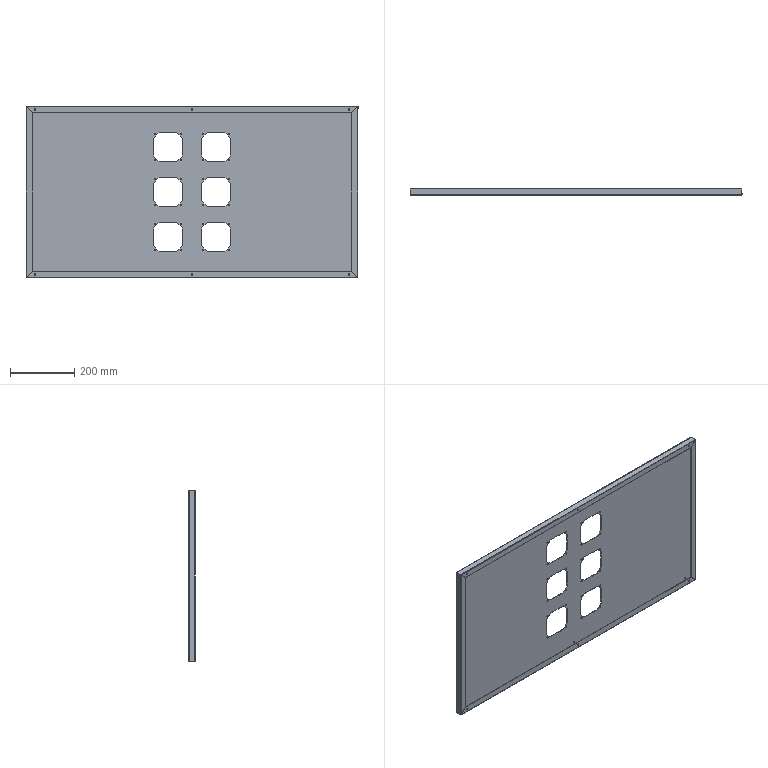Part | SolidWorks | features SplitBody 1 | 1 solid | 190 faces | box 1035 x 20 x 535 mm | volume 624346 mm3 | cylinder 112 | plane 62 | spline 16 | commonest cylinder face diameters 4.5 x72 105 x24 0.2 x8 2.2 x8